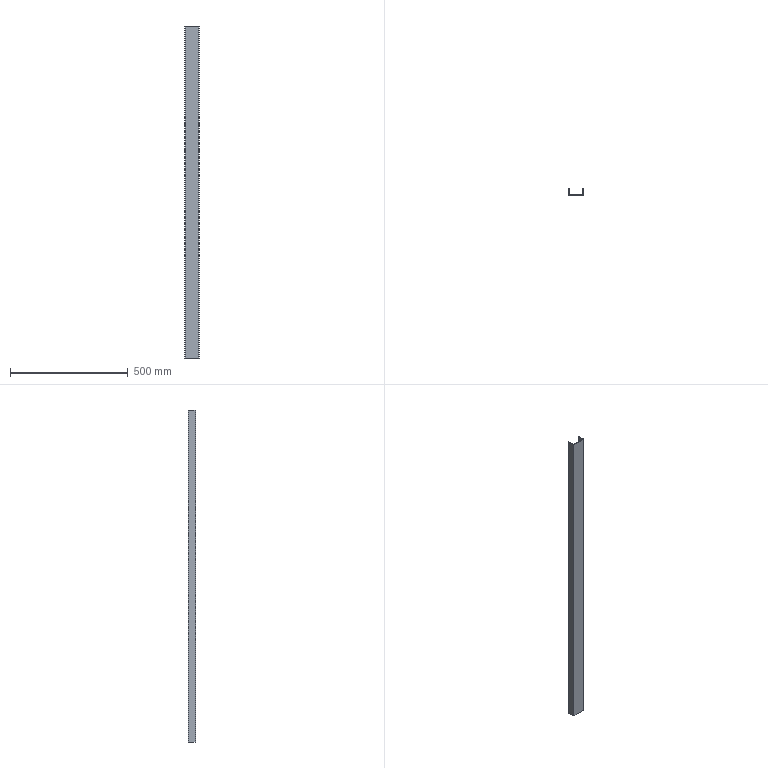Part | STEP file | Guard Stiffening Rib | 1 solid | 14 faces | box 60 x 30 x 1408 mm | volume 244838 mm3 | plane 10 | cylinder 4 | commonest cylinder face diameters 1 x2 4 x2
STEP:
#1=CARTESIAN_POINT('',(37.268,-14.819,1408.));
#2=VERTEX_POINT('',#1);
#3=CARTESIAN_POINT('',(93.268,-14.819,1408.));
#4=VERTEX_POINT('',#3);
#5=CARTESIAN_POINT('',(35.268,-14.819,1408.));
#6=DIRECTION('',(1.,0.,0.));
#7=VECTOR('',#6,1000.);
#8=LINE('',#5,#7);
#9=EDGE_CURVE('',#2,#4,#8,.T.);
#10=ORIENTED_EDGE('',*,*,#9,.T.);
#11=CARTESIAN_POINT('',(93.268,-14.819,0.));
#12=VERTEX_POINT('',#11);
#13=CARTESIAN_POINT('',(93.268,-14.819,1408.));
#14=DIRECTION('',(0.,0.,-1.));
#15=VECTOR('',#14,1000.);
#16=LINE('',#13,#15);
#17=EDGE_CURVE('',#4,#12,#16,.T.);
#18=ORIENTED_EDGE('',*,*,#17,.T.);
#19=CARTESIAN_POINT('',(37.268,-14.819,0.));
#20=VERTEX_POINT('',#19);
#21=CARTESIAN_POINT('',(35.268,-14.819,0.));
#22=DIRECTION('',(-1.,0.,0.));
#23=VECTOR('',#22,1000.);
#24=LINE('',#21,#23);
#25=EDGE_CURVE('',#12,#20,#24,.T.);
#26=ORIENTED_EDGE('',*,*,#25,.T.);
#27=CARTESIAN_POINT('',(37.268,-14.819,1408.));
#28=DIRECTION('',(0.,0.,1.));
#29=VECTOR('',#28,1000.);
#30=LINE('',#27,#29);
#31=EDGE_CURVE('',#20,#2,#30,.T.);
#32=ORIENTED_EDGE('',*,*,#31,.T.);
#33=EDGE_LOOP('',(#10,#18,#26,#32));
#34=FACE_OUTER_BOUND('',#33,.T.);
#35=CARTESIAN_POINT('',(35.268,-14.819,1408.));
#36=DIRECTION('',(0.,1.,0.));
#37=DIRECTION('',(0.,0.,1.));
#38=AXIS2_PLACEMENT_3D('',#35,#36,#37);
#39=PLANE('',#38);
#40=ADVANCED_FACE('',(#34),#39,.T.);
#41=ORIENTED_EDGE('',*,*,#17,.F.);
#42=CARTESIAN_POINT('',(93.768,-14.319,1408.));
#43=VERTEX_POINT('',#42);
#44=CARTESIAN_POINT('',(93.268,-14.319,1408.));
#45=DIRECTION('',(0.,0.,-1.));
#46=DIRECTION('',(-1.,0.,0.));
#47=AXIS2_PLACEMENT_3D('',#44,#45,#46);
#48=CIRCLE('',#47,0.5);
#49=EDGE_CURVE('',#43,#4,#48,.T.);
#50=ORIENTED_EDGE('',*,*,#49,.F.);
#51=CARTESIAN_POINT('',(93.768,-14.319,0.));
#52=VERTEX_POINT('',#51);
#53=CARTESIAN_POINT('',(93.768,-14.319,1408.));
#54=DIRECTION('',(0.,0.,1.));
#55=VECTOR('',#54,1000.);
#56=LINE('',#53,#55);
#57=EDGE_CURVE('',#52,#43,#56,.T.);
#58=ORIENTED_EDGE('',*,*,#57,.F.);
#59=CARTESIAN_POINT('',(93.268,-14.319,0.));
#60=DIRECTION('',(0.,0.,1.));
#61=DIRECTION('',(-1.,0.,0.));
#62=AXIS2_PLACEMENT_3D('',#59,#60,#61);
#63=CIRCLE('',#62,0.5);
#64=EDGE_CURVE('',#12,#52,#63,.T.);
#65=ORIENTED_EDGE('',*,*,#64,.F.);
#66=EDGE_LOOP('',(#41,#50,#58,#65));
#67=FACE_OUTER_BOUND('',#66,.T.);
#68=CARTESIAN_POINT('',(93.268,-14.319,1408.));
#69=DIRECTION('',(0.,0.,-1.));
#70=DIRECTION('',(-1.,0.,0.));
#71=AXIS2_PLACEMENT_3D('',#68,#69,#70);
#72=CYLINDRICAL_SURFACE('',#71,0.5);
#73=ADVANCED_FACE('',(#67),#72,.F.);
#74=ORIENTED_EDGE('',*,*,#9,.F.);
#75=CARTESIAN_POINT('',(36.768,-14.319,1408.));
#76=VERTEX_POINT('',#75);
#77=CARTESIAN_POINT('',(37.268,-14.319,1408.));
#78=DIRECTION('',(0.,0.,-1.));
#79=DIRECTION('',(-1.,0.,0.));
#80=AXIS2_PLACEMENT_3D('',#77,#78,#79);
#81=CIRCLE('',#80,0.5);
#82=EDGE_CURVE('',#2,#76,#81,.T.);
#83=ORIENTED_EDGE('',*,*,#82,.T.);
#84=CARTESIAN_POINT('',(36.768,13.681,1408.));
#85=VERTEX_POINT('',#84);
#86=CARTESIAN_POINT('',(36.768,13.681,1408.));
#87=DIRECTION('',(0.,-1.,0.));
#88=VECTOR('',#87,1000.);
#89=LINE('',#86,#88);
#90=EDGE_CURVE('',#85,#76,#89,.T.);
#91=ORIENTED_EDGE('',*,*,#90,.F.);
#92=CARTESIAN_POINT('',(35.268,13.681,1408.));
#93=VERTEX_POINT('',#92);
#94=CARTESIAN_POINT('',(37.268,13.681,1408.));
#95=DIRECTION('',(-1.,0.,0.));
#96=VECTOR('',#95,1000.);
#97=LINE('',#94,#96);
#98=EDGE_CURVE('',#85,#93,#97,.T.);
#99=ORIENTED_EDGE('',*,*,#98,.T.);
#100=CARTESIAN_POINT('',(35.268,-14.319,1408.));
#101=VERTEX_POINT('',#100);
#102=CARTESIAN_POINT('',(35.268,-14.819,1408.));
#103=DIRECTION('',(0.,-1.,0.));
#104=VECTOR('',#103,1000.);
#105=LINE('',#102,#104);
#106=EDGE_CURVE('',#93,#101,#105,.T.);
#107=ORIENTED_EDGE('',*,*,#106,.T.);
#108=CARTESIAN_POINT('',(37.268,-16.319,1408.));
#109=VERTEX_POINT('',#108);
#110=CARTESIAN_POINT('',(37.268,-14.319,1408.));
#111=DIRECTION('',(0.,0.,-1.));
#112=DIRECTION('',(-1.,0.,0.));
#113=AXIS2_PLACEMENT_3D('',#110,#111,#112);
#114=CIRCLE('',#113,2.);
#115=EDGE_CURVE('',#109,#101,#114,.T.);
#116=ORIENTED_EDGE('',*,*,#115,.F.);
#117=CARTESIAN_POINT('',(93.268,-16.319,1408.));
#118=VERTEX_POINT('',#117);
#119=CARTESIAN_POINT('',(93.768,-16.319,1408.));
#120=DIRECTION('',(1.,0.,0.));
#121=VECTOR('',#120,1000.);
#122=LINE('',#119,#121);
#123=EDGE_CURVE('',#109,#118,#122,.T.);
#124=ORIENTED_EDGE('',*,*,#123,.T.);
#125=CARTESIAN_POINT('',(95.268,-14.319,1408.));
#126=VERTEX_POINT('',#125);
#127=CARTESIAN_POINT('',(93.268,-14.319,1408.));
#128=DIRECTION('',(0.,0.,-1.));
#129=DIRECTION('',(-1.,0.,0.));
#130=AXIS2_PLACEMENT_3D('',#127,#128,#129);
#131=CIRCLE('',#130,2.);
#132=EDGE_CURVE('',#126,#118,#131,.T.);
#133=ORIENTED_EDGE('',*,*,#132,.F.);
#134=CARTESIAN_POINT('',(95.268,13.681,1408.));
#135=VERTEX_POINT('',#134);
#136=CARTESIAN_POINT('',(95.268,-14.319,1408.));
#137=DIRECTION('',(0.,1.,0.));
#138=VECTOR('',#137,1000.);
#139=LINE('',#136,#138);
#140=EDGE_CURVE('',#126,#135,#139,.T.);
#141=ORIENTED_EDGE('',*,*,#140,.T.);
#142=CARTESIAN_POINT('',(93.768,13.681,1408.));
#143=VERTEX_POINT('',#142);
#144=CARTESIAN_POINT('',(93.768,13.681,1408.));
#145=DIRECTION('',(1.,0.,0.));
#146=VECTOR('',#145,1000.);
#147=LINE('',#144,#146);
#148=EDGE_CURVE('',#143,#135,#147,.T.);
#149=ORIENTED_EDGE('',*,*,#148,.F.);
#150=CARTESIAN_POINT('',(93.768,-16.319,1408.));
#151=DIRECTION('',(0.,1.,0.));
#152=VECTOR('',#151,1000.);
#153=LINE('',#150,#152);
#154=EDGE_CURVE('',#43,#143,#153,.T.);
#155=ORIENTED_EDGE('',*,*,#154,.F.);
#156=ORIENTED_EDGE('',*,*,#49,.T.);
#157=EDGE_LOOP('',(#74,#83,#91,#99,#107,#116,#124,#133,#141,#149,#155,#156));
#158=FACE_OUTER_BOUND('',#157,.T.);
#159=CARTESIAN_POINT('',(93.768,-14.319,1408.));
#160=DIRECTION('',(0.,0.,1.));
#161=DIRECTION('',(1.,0.,0.));
#162=AXIS2_PLACEMENT_3D('',#159,#160,#161);
#163=PLANE('',#162);
#164=ADVANCED_FACE('',(#158),#163,.T.);
#165=CARTESIAN_POINT('',(36.768,-14.319,0.));
#166=VERTEX_POINT('',#165);
#167=CARTESIAN_POINT('',(36.768,-14.319,1408.));
#168=DIRECTION('',(0.,0.,-1.));
#169=VECTOR('',#168,1000.);
#170=LINE('',#167,#169);
#171=EDGE_CURVE('',#76,#166,#170,.T.);
#172=ORIENTED_EDGE('',*,*,#171,.F.);
#173=ORIENTED_EDGE('',*,*,#82,.F.);
#174=ORIENTED_EDGE('',*,*,#31,.F.);
#175=CARTESIAN_POINT('',(37.268,-14.319,0.));
#176=DIRECTION('',(0.,0.,1.));
#177=DIRECTION('',(-1.,0.,0.));
#178=AXIS2_PLACEMENT_3D('',#175,#176,#177);
#179=CIRCLE('',#178,0.5);
#180=EDGE_CURVE('',#166,#20,#179,.T.);
#181=ORIENTED_EDGE('',*,*,#180,.F.);
#182=EDGE_LOOP('',(#172,#173,#174,#181));
#183=FACE_OUTER_BOUND('',#182,.T.);
#184=CARTESIAN_POINT('',(37.268,-14.319,1408.));
#185=DIRECTION('',(0.,0.,-1.));
#186=DIRECTION('',(-1.,0.,0.));
#187=AXIS2_PLACEMENT_3D('',#184,#185,#186);
#188=CYLINDRICAL_SURFACE('',#187,0.5);
#189=ADVANCED_FACE('',(#183),#188,.F.);
#190=ORIENTED_EDGE('',*,*,#25,.F.);
#191=ORIENTED_EDGE('',*,*,#64,.T.);
#192=CARTESIAN_POINT('',(93.768,13.681,0.));
#193=VERTEX_POINT('',#192);
#194=CARTESIAN_POINT('',(93.768,-16.319,0.));
#195=DIRECTION('',(0.,-1.,0.));
#196=VECTOR('',#195,1000.);
#197=LINE('',#194,#196);
#198=EDGE_CURVE('',#193,#52,#197,.T.);
#199=ORIENTED_EDGE('',*,*,#198,.F.);
#200=CARTESIAN_POINT('',(95.268,13.681,0.));
#201=VERTEX_POINT('',#200);
#202=CARTESIAN_POINT('',(93.768,13.681,0.));
#203=DIRECTION('',(-1.,0.,0.));
#204=VECTOR('',#203,1000.);
#205=LINE('',#202,#204);
#206=EDGE_CURVE('',#201,#193,#205,.T.);
#207=ORIENTED_EDGE('',*,*,#206,.F.);
#208=CARTESIAN_POINT('',(95.268,-14.319,0.));
#209=VERTEX_POINT('',#208);
#210=CARTESIAN_POINT('',(95.268,-14.819,0.));
#211=DIRECTION('',(0.,-1.,0.));
#212=VECTOR('',#211,1000.);
#213=LINE('',#210,#212);
#214=EDGE_CURVE('',#201,#209,#213,.T.);
#215=ORIENTED_EDGE('',*,*,#214,.T.);
#216=CARTESIAN_POINT('',(93.268,-16.319,0.));
#217=VERTEX_POINT('',#216);
#218=CARTESIAN_POINT('',(93.268,-14.319,0.));
#219=DIRECTION('',(0.,0.,1.));
#220=DIRECTION('',(-1.,0.,0.));
#221=AXIS2_PLACEMENT_3D('',#218,#219,#220);
#222=CIRCLE('',#221,2.);
#223=EDGE_CURVE('',#217,#209,#222,.T.);
#224=ORIENTED_EDGE('',*,*,#223,.F.);
#225=CARTESIAN_POINT('',(37.268,-16.319,0.));
#226=VERTEX_POINT('',#225);
#227=CARTESIAN_POINT('',(36.768,-16.319,0.));
#228=DIRECTION('',(-1.,0.,0.));
#229=VECTOR('',#228,1000.);
#230=LINE('',#227,#229);
#231=EDGE_CURVE('',#217,#226,#230,.T.);
#232=ORIENTED_EDGE('',*,*,#231,.T.);
#233=CARTESIAN_POINT('',(35.268,-14.319,0.));
#234=VERTEX_POINT('',#233);
#235=CARTESIAN_POINT('',(37.268,-14.319,0.));
#236=DIRECTION('',(0.,0.,1.));
#237=DIRECTION('',(-1.,0.,0.));
#238=AXIS2_PLACEMENT_3D('',#235,#236,#237);
#239=CIRCLE('',#238,2.);
#240=EDGE_CURVE('',#234,#226,#239,.T.);
#241=ORIENTED_EDGE('',*,*,#240,.F.);
#242=CARTESIAN_POINT('',(35.268,13.681,0.));
#243=VERTEX_POINT('',#242);
#244=CARTESIAN_POINT('',(35.268,-14.319,0.));
#245=DIRECTION('',(0.,-1.,0.));
#246=VECTOR('',#245,1000.);
#247=LINE('',#244,#246);
#248=EDGE_CURVE('',#243,#234,#247,.T.);
#249=ORIENTED_EDGE('',*,*,#248,.F.);
#250=CARTESIAN_POINT('',(36.768,13.681,0.));
#251=VERTEX_POINT('',#250);
#252=CARTESIAN_POINT('',(35.268,13.681,0.));
#253=DIRECTION('',(-1.,0.,0.));
#254=VECTOR('',#253,1000.);
#255=LINE('',#252,#254);
#256=EDGE_CURVE('',#251,#243,#255,.T.);
#257=ORIENTED_EDGE('',*,*,#256,.F.);
#258=CARTESIAN_POINT('',(36.768,13.681,0.));
#259=DIRECTION('',(0.,1.,0.));
#260=VECTOR('',#259,1000.);
#261=LINE('',#258,#260);
#262=EDGE_CURVE('',#166,#251,#261,.T.);
#263=ORIENTED_EDGE('',*,*,#262,.F.);
#264=ORIENTED_EDGE('',*,*,#180,.T.);
#265=EDGE_LOOP('',(#190,#191,#199,#207,#215,#224,#232,#241,#249,#257,#263,#264));
#266=FACE_OUTER_BOUND('',#265,.T.);
#267=CARTESIAN_POINT('',(36.768,-14.319,0.));
#268=DIRECTION('',(0.,0.,-1.));
#269=DIRECTION('',(-1.,0.,0.));
#270=AXIS2_PLACEMENT_3D('',#267,#268,#269);
#271=PLANE('',#270);
#272=ADVANCED_FACE('',(#266),#271,.T.);
#273=ORIENTED_EDGE('',*,*,#154,.T.);
#274=CARTESIAN_POINT('',(93.768,13.681,1408.));
#275=DIRECTION('',(0.,0.,-1.));
#276=VECTOR('',#275,1000.);
#277=LINE('',#274,#276);
#278=EDGE_CURVE('',#143,#193,#277,.T.);
#279=ORIENTED_EDGE('',*,*,#278,.T.);
#280=ORIENTED_EDGE('',*,*,#198,.T.);
#281=ORIENTED_EDGE('',*,*,#57,.T.);
#282=EDGE_LOOP('',(#273,#279,#280,#281));
#283=FACE_OUTER_BOUND('',#282,.T.);
#284=CARTESIAN_POINT('',(93.768,-16.319,1408.));
#285=DIRECTION('',(-1.,0.,0.));
#286=DIRECTION('',(0.,0.,1.));
#287=AXIS2_PLACEMENT_3D('',#284,#285,#286);
#288=PLANE('',#287);
#289=ADVANCED_FACE('',(#283),#288,.T.);
#290=CARTESIAN_POINT('',(93.268,-16.319,1408.));
#291=DIRECTION('',(0.,0.,-1.));
#292=VECTOR('',#291,1000.);
#293=LINE('',#290,#292);
#294=EDGE_CURVE('',#118,#217,#293,.T.);
#295=ORIENTED_EDGE('',*,*,#294,.F.);
#296=ORIENTED_EDGE('',*,*,#123,.F.);
#297=CARTESIAN_POINT('',(37.268,-16.319,1408.));
#298=DIRECTION('',(0.,0.,1.));
#299=VECTOR('',#298,1000.);
#300=LINE('',#297,#299);
#301=EDGE_CURVE('',#226,#109,#300,.T.);
#302=ORIENTED_EDGE('',*,*,#301,.F.);
#303=ORIENTED_EDGE('',*,*,#231,.F.);
#304=EDGE_LOOP('',(#295,#296,#302,#303));
#305=FACE_OUTER_BOUND('',#304,.T.);
#306=CARTESIAN_POINT('',(35.268,-16.319,1408.));
#307=DIRECTION('',(0.,1.,0.));
#308=DIRECTION('',(0.,0.,1.));
#309=AXIS2_PLACEMENT_3D('',#306,#307,#308);
#310=PLANE('',#309);
#311=ADVANCED_FACE('',(#305),#310,.F.);
#312=ORIENTED_EDGE('',*,*,#90,.T.);
#313=ORIENTED_EDGE('',*,*,#171,.T.);
#314=ORIENTED_EDGE('',*,*,#262,.T.);
#315=CARTESIAN_POINT('',(36.768,13.681,1408.));
#316=DIRECTION('',(0.,0.,1.));
#317=VECTOR('',#316,1000.);
#318=LINE('',#315,#317);
#319=EDGE_CURVE('',#251,#85,#318,.T.);
#320=ORIENTED_EDGE('',*,*,#319,.T.);
#321=EDGE_LOOP('',(#312,#313,#314,#320));
#322=FACE_OUTER_BOUND('',#321,.T.);
#323=CARTESIAN_POINT('',(36.768,13.681,1408.));
#324=DIRECTION('',(1.,0.,0.));
#325=DIRECTION('',(0.,0.,-1.));
#326=AXIS2_PLACEMENT_3D('',#323,#324,#325);
#327=PLANE('',#326);
#328=ADVANCED_FACE('',(#322),#327,.T.);
#329=ORIENTED_EDGE('',*,*,#148,.T.);
#330=CARTESIAN_POINT('',(95.268,13.681,1408.));
#331=DIRECTION('',(0.,0.,-1.));
#332=VECTOR('',#331,1000.);
#333=LINE('',#330,#332);
#334=EDGE_CURVE('',#135,#201,#333,.T.);
#335=ORIENTED_EDGE('',*,*,#334,.T.);
#336=ORIENTED_EDGE('',*,*,#206,.T.);
#337=ORIENTED_EDGE('',*,*,#278,.F.);
#338=EDGE_LOOP('',(#329,#335,#336,#337));
#339=FACE_OUTER_BOUND('',#338,.T.);
#340=CARTESIAN_POINT('',(93.768,13.681,1408.));
#341=DIRECTION('',(0.,1.,0.));
#342=DIRECTION('',(0.,0.,1.));
#343=AXIS2_PLACEMENT_3D('',#340,#341,#342);
#344=PLANE('',#343);
#345=ADVANCED_FACE('',(#339),#344,.T.);
#346=ORIENTED_EDGE('',*,*,#132,.T.);
#347=ORIENTED_EDGE('',*,*,#294,.T.);
#348=ORIENTED_EDGE('',*,*,#223,.T.);
#349=CARTESIAN_POINT('',(95.268,-14.319,1408.));
#350=DIRECTION('',(0.,0.,1.));
#351=VECTOR('',#350,1000.);
#352=LINE('',#349,#351);
#353=EDGE_CURVE('',#209,#126,#352,.T.);
#354=ORIENTED_EDGE('',*,*,#353,.T.);
#355=EDGE_LOOP('',(#346,#347,#348,#354));
#356=FACE_OUTER_BOUND('',#355,.T.);
#357=CARTESIAN_POINT('',(93.268,-14.319,1408.));
#358=DIRECTION('',(0.,0.,-1.));
#359=DIRECTION('',(-1.,0.,0.));
#360=AXIS2_PLACEMENT_3D('',#357,#358,#359);
#361=CYLINDRICAL_SURFACE('',#360,2.);
#362=ADVANCED_FACE('',(#356),#361,.T.);
#363=ORIENTED_EDGE('',*,*,#115,.T.);
#364=CARTESIAN_POINT('',(35.268,-14.319,1408.));
#365=DIRECTION('',(0.,0.,-1.));
#366=VECTOR('',#365,1000.);
#367=LINE('',#364,#366);
#368=EDGE_CURVE('',#101,#234,#367,.T.);
#369=ORIENTED_EDGE('',*,*,#368,.T.);
#370=ORIENTED_EDGE('',*,*,#240,.T.);
#371=ORIENTED_EDGE('',*,*,#301,.T.);
#372=EDGE_LOOP('',(#363,#369,#370,#371));
#373=FACE_OUTER_BOUND('',#372,.T.);
#374=CARTESIAN_POINT('',(37.268,-14.319,1408.));
#375=DIRECTION('',(0.,0.,-1.));
#376=DIRECTION('',(-1.,0.,0.));
#377=AXIS2_PLACEMENT_3D('',#374,#375,#376);
#378=CYLINDRICAL_SURFACE('',#377,2.);
#379=ADVANCED_FACE('',(#373),#378,.T.);
#380=ORIENTED_EDGE('',*,*,#98,.F.);
#381=ORIENTED_EDGE('',*,*,#319,.F.);
#382=ORIENTED_EDGE('',*,*,#256,.T.);
#383=CARTESIAN_POINT('',(35.268,13.681,1408.));
#384=DIRECTION('',(0.,0.,1.));
#385=VECTOR('',#384,1000.);
#386=LINE('',#383,#385);
#387=EDGE_CURVE('',#243,#93,#386,.T.);
#388=ORIENTED_EDGE('',*,*,#387,.T.);
#389=EDGE_LOOP('',(#380,#381,#382,#388));
#390=FACE_OUTER_BOUND('',#389,.T.);
#391=CARTESIAN_POINT('',(35.268,13.681,1408.));
#392=DIRECTION('',(0.,1.,0.));
#393=DIRECTION('',(0.,0.,1.));
#394=AXIS2_PLACEMENT_3D('',#391,#392,#393);
#395=PLANE('',#394);
#396=ADVANCED_FACE('',(#390),#395,.T.);
#397=ORIENTED_EDGE('',*,*,#334,.F.);
#398=ORIENTED_EDGE('',*,*,#140,.F.);
#399=ORIENTED_EDGE('',*,*,#353,.F.);
#400=ORIENTED_EDGE('',*,*,#214,.F.);
#401=EDGE_LOOP('',(#397,#398,#399,#400));
#402=FACE_OUTER_BOUND('',#401,.T.);
#403=CARTESIAN_POINT('',(95.268,-16.319,1408.));
#404=DIRECTION('',(-1.,0.,0.));
#405=DIRECTION('',(0.,0.,1.));
#406=AXIS2_PLACEMENT_3D('',#403,#404,#405);
#407=PLANE('',#406);
#408=ADVANCED_FACE('',(#402),#407,.F.);
#409=ORIENTED_EDGE('',*,*,#368,.F.);
#410=ORIENTED_EDGE('',*,*,#106,.F.);
#411=ORIENTED_EDGE('',*,*,#387,.F.);
#412=ORIENTED_EDGE('',*,*,#248,.T.);
#413=EDGE_LOOP('',(#409,#410,#411,#412));
#414=FACE_OUTER_BOUND('',#413,.T.);
#415=CARTESIAN_POINT('',(35.268,13.681,1408.));
#416=DIRECTION('',(1.,0.,0.));
#417=DIRECTION('',(0.,0.,-1.));
#418=AXIS2_PLACEMENT_3D('',#415,#416,#417);
#419=PLANE('',#418);
#420=ADVANCED_FACE('',(#414),#419,.F.);
#421=CLOSED_SHELL('',(#40,#73,#164,#189,#272,#289,#311,#328,#345,#362,#379,#396,#408,#420));
#422=MANIFOLD_SOLID_BREP('',#421);
#423=CARTESIAN_POINT('',(0.,0.,0.));
#424=DIRECTION('',(0.,0.,1.));
#425=DIRECTION('',(1.,0.,0.));
#426=AXIS2_PLACEMENT_3D('',#423,#424,#425);
#427=(LENGTH_UNIT()NAMED_UNIT(*)SI_UNIT(.MILLI.,.METRE.));
#428=UNCERTAINTY_MEASURE_WITH_UNIT(LENGTH_MEASURE(0.00001),#427,'','');
#429=(NAMED_UNIT(*)PLANE_ANGLE_UNIT()SI_UNIT($,.RADIAN.));
#430=(NAMED_UNIT(*)SI_UNIT($,.STERADIAN.)SOLID_ANGLE_UNIT());
#431=(GEOMETRIC_REPRESENTATION_CONTEXT(3)GLOBAL_UNCERTAINTY_ASSIGNED_CONTEXT((#428))GLOBAL_UNIT_ASSIGNED_CONTEXT((#427,#429,#430))REPRESENTATION_CONTEXT('',''));
#432=ADVANCED_BREP_SHAPE_REPRESENTATION('',(#422,#426),#431);